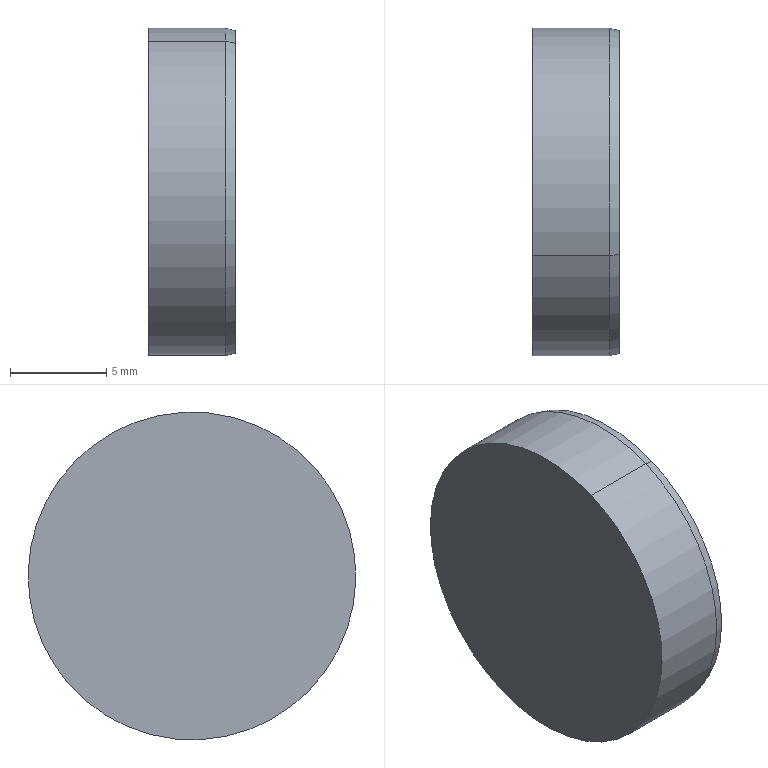Part | SolidWorks | features BaseBody 1 | 1 solid | 6 faces | box 4.5 x 17 x 17 mm | volume 1020 mm3 | cylinder 2 | cone 2 | plane 2 | commonest cylinder face diameters 17 x2
STEP:
#1=CARTESIAN_POINT('',(-85.763,-1.409,-188.719));
#2=VERTEX_POINT('',#1);
#3=CARTESIAN_POINT('',(-85.763,5.202,-204.381));
#4=VERTEX_POINT('',#3);
#5=CARTESIAN_POINT('',(-85.763,1.896,-196.55));
#6=DIRECTION('',(-1.,0.,0.));
#7=DIRECTION('',(0.,0.3889,-0.9213));
#8=AXIS2_PLACEMENT_3D('',#5,#6,#7);
#9=CIRCLE('',#8,8.5);
#10=EDGE_CURVE('',#2,#4,#9,.T.);
#11=ORIENTED_EDGE('',*,*,#10,.T.);
#12=CARTESIAN_POINT('',(-89.763,5.202,-204.381));
#13=VERTEX_POINT('',#12);
#14=CARTESIAN_POINT('',(-85.263,5.202,-204.381));
#15=DIRECTION('',(-1.,0.,0.));
#16=VECTOR('',#15,1000.);
#17=LINE('',#14,#16);
#18=EDGE_CURVE('',#4,#13,#17,.T.);
#19=ORIENTED_EDGE('',*,*,#18,.T.);
#20=CARTESIAN_POINT('',(-89.763,-1.409,-188.719));
#21=VERTEX_POINT('',#20);
#22=CARTESIAN_POINT('',(-89.763,1.896,-196.55));
#23=DIRECTION('',(1.,0.,0.));
#24=DIRECTION('',(0.,0.3889,-0.9213));
#25=AXIS2_PLACEMENT_3D('',#22,#23,#24);
#26=CIRCLE('',#25,8.5);
#27=EDGE_CURVE('',#13,#21,#26,.T.);
#28=ORIENTED_EDGE('',*,*,#27,.T.);
#29=CARTESIAN_POINT('',(-85.263,-1.409,-188.719));
#30=DIRECTION('',(-1.,0.,0.));
#31=VECTOR('',#30,1000.);
#32=LINE('',#29,#31);
#33=EDGE_CURVE('',#2,#21,#32,.T.);
#34=ORIENTED_EDGE('',*,*,#33,.F.);
#35=EDGE_LOOP('',(#11,#19,#28,#34));
#36=FACE_OUTER_BOUND('',#35,.T.);
#37=CARTESIAN_POINT('',(-85.263,1.896,-196.55));
#38=DIRECTION('',(-1.,0.,0.));
#39=DIRECTION('',(0.,-0.3889,0.9213));
#40=AXIS2_PLACEMENT_3D('',#37,#38,#39);
#41=CYLINDRICAL_SURFACE('',#40,8.5);
#42=ADVANCED_FACE('',(#36),#41,.T.);
#43=CARTESIAN_POINT('',(-85.263,5.15,-204.258));
#44=VERTEX_POINT('',#43);
#45=CARTESIAN_POINT('',(-85.263,-1.357,-188.842));
#46=VERTEX_POINT('',#45);
#47=CARTESIAN_POINT('',(-85.263,1.896,-196.55));
#48=DIRECTION('',(1.,0.,0.));
#49=DIRECTION('',(0.,0.3889,-0.9213));
#50=AXIS2_PLACEMENT_3D('',#47,#48,#49);
#51=CIRCLE('',#50,8.366);
#52=EDGE_CURVE('',#44,#46,#51,.T.);
#53=ORIENTED_EDGE('',*,*,#52,.F.);
#54=CARTESIAN_POINT('',(-85.263,5.15,-204.258));
#55=DIRECTION('',(-0.9659,0.1007,-0.2384));
#56=VECTOR('',#55,1000.);
#57=LINE('',#54,#56);
#58=EDGE_CURVE('',#44,#4,#57,.T.);
#59=ORIENTED_EDGE('',*,*,#58,.T.);
#60=ORIENTED_EDGE('',*,*,#10,.F.);
#61=CARTESIAN_POINT('',(-85.263,-1.357,-188.842));
#62=DIRECTION('',(-0.9659,-0.1007,0.2384));
#63=VECTOR('',#62,1000.);
#64=LINE('',#61,#63);
#65=EDGE_CURVE('',#46,#2,#64,.T.);
#66=ORIENTED_EDGE('',*,*,#65,.F.);
#67=EDGE_LOOP('',(#53,#59,#60,#66));
#68=FACE_OUTER_BOUND('',#67,.T.);
#69=CARTESIAN_POINT('',(-85.263,1.896,-196.55));
#70=DIRECTION('',(-1.,0.,0.));
#71=DIRECTION('',(0.,-0.3889,0.9213));
#72=AXIS2_PLACEMENT_3D('',#69,#70,#71);
#73=CONICAL_SURFACE('',#72,8.366,0.2618);
#74=ADVANCED_FACE('',(#68),#73,.T.);
#75=ORIENTED_EDGE('',*,*,#58,.F.);
#76=CARTESIAN_POINT('',(-85.263,1.896,-196.55));
#77=DIRECTION('',(1.,0.,0.));
#78=DIRECTION('',(0.,0.3889,-0.9213));
#79=AXIS2_PLACEMENT_3D('',#76,#77,#78);
#80=CIRCLE('',#79,8.366);
#81=EDGE_CURVE('',#46,#44,#80,.T.);
#82=ORIENTED_EDGE('',*,*,#81,.F.);
#83=ORIENTED_EDGE('',*,*,#65,.T.);
#84=CARTESIAN_POINT('',(-85.763,1.896,-196.55));
#85=DIRECTION('',(-1.,0.,0.));
#86=DIRECTION('',(0.,0.3889,-0.9213));
#87=AXIS2_PLACEMENT_3D('',#84,#85,#86);
#88=CIRCLE('',#87,8.5);
#89=EDGE_CURVE('',#4,#2,#88,.T.);
#90=ORIENTED_EDGE('',*,*,#89,.F.);
#91=EDGE_LOOP('',(#75,#82,#83,#90));
#92=FACE_OUTER_BOUND('',#91,.T.);
#93=CARTESIAN_POINT('',(-85.263,1.896,-196.55));
#94=DIRECTION('',(-1.,0.,0.));
#95=DIRECTION('',(0.,-0.3889,0.9213));
#96=AXIS2_PLACEMENT_3D('',#93,#94,#95);
#97=CONICAL_SURFACE('',#96,8.366,0.2618);
#98=ADVANCED_FACE('',(#92),#97,.T.);
#99=CARTESIAN_POINT('',(-89.763,1.896,-196.55));
#100=DIRECTION('',(1.,0.,0.));
#101=DIRECTION('',(0.,0.3889,-0.9213));
#102=AXIS2_PLACEMENT_3D('',#99,#100,#101);
#103=CIRCLE('',#102,8.5);
#104=EDGE_CURVE('',#21,#13,#103,.T.);
#105=ORIENTED_EDGE('',*,*,#104,.F.);
#106=ORIENTED_EDGE('',*,*,#27,.F.);
#107=EDGE_LOOP('',(#105,#106));
#108=FACE_OUTER_BOUND('',#107,.T.);
#109=CARTESIAN_POINT('',(-89.763,1.896,-196.55));
#110=DIRECTION('',(1.,0.,0.));
#111=DIRECTION('',(0.,0.,-1.));
#112=AXIS2_PLACEMENT_3D('',#109,#110,#111);
#113=PLANE('',#112);
#114=ADVANCED_FACE('',(#108),#113,.F.);
#115=ORIENTED_EDGE('',*,*,#81,.T.);
#116=ORIENTED_EDGE('',*,*,#52,.T.);
#117=EDGE_LOOP('',(#115,#116));
#118=FACE_OUTER_BOUND('',#117,.T.);
#119=CARTESIAN_POINT('',(-85.263,1.896,-196.55));
#120=DIRECTION('',(1.,0.,0.));
#121=DIRECTION('',(0.,0.,-1.));
#122=AXIS2_PLACEMENT_3D('',#119,#120,#121);
#123=PLANE('',#122);
#124=ADVANCED_FACE('',(#118),#123,.T.);
#125=ORIENTED_EDGE('',*,*,#18,.F.);
#126=ORIENTED_EDGE('',*,*,#89,.T.);
#127=ORIENTED_EDGE('',*,*,#33,.T.);
#128=ORIENTED_EDGE('',*,*,#104,.T.);
#129=EDGE_LOOP('',(#125,#126,#127,#128));
#130=FACE_OUTER_BOUND('',#129,.T.);
#131=CARTESIAN_POINT('',(-85.263,1.896,-196.55));
#132=DIRECTION('',(-1.,0.,0.));
#133=DIRECTION('',(0.,-0.3889,0.9213));
#134=AXIS2_PLACEMENT_3D('',#131,#132,#133);
#135=CYLINDRICAL_SURFACE('',#134,8.5);
#136=ADVANCED_FACE('',(#130),#135,.T.);
#137=CLOSED_SHELL('',(#42,#74,#98,#114,#124,#136));
#138=MANIFOLD_SOLID_BREP('',#137);
#139=CARTESIAN_POINT('',(0.,0.,0.));
#140=DIRECTION('',(0.,0.,1.));
#141=DIRECTION('',(1.,0.,0.));
#142=AXIS2_PLACEMENT_3D('',#139,#140,#141);
#143=(LENGTH_UNIT()NAMED_UNIT(*)SI_UNIT(.MILLI.,.METRE.));
#144=UNCERTAINTY_MEASURE_WITH_UNIT(LENGTH_MEASURE(0.00001),#143,'','');
#145=(NAMED_UNIT(*)PLANE_ANGLE_UNIT()SI_UNIT($,.RADIAN.));
#146=(NAMED_UNIT(*)SI_UNIT($,.STERADIAN.)SOLID_ANGLE_UNIT());
#147=(GEOMETRIC_REPRESENTATION_CONTEXT(3)GLOBAL_UNCERTAINTY_ASSIGNED_CONTEXT((#144))GLOBAL_UNIT_ASSIGNED_CONTEXT((#143,#145,#146))REPRESENTATION_CONTEXT('',''));
#148=ADVANCED_BREP_SHAPE_REPRESENTATION('',(#138,#142),#147);